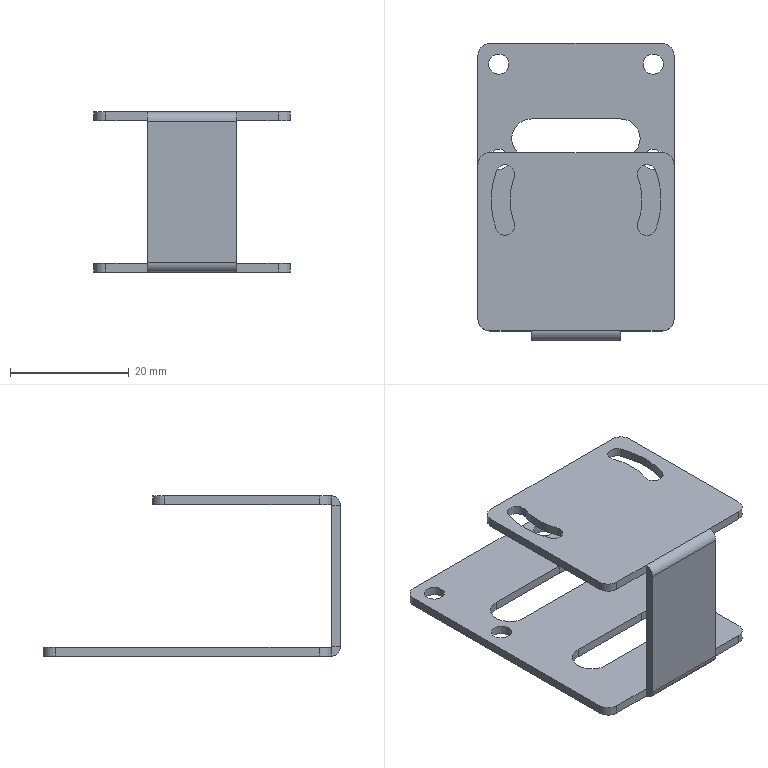Part | STEP file | 1 solid | 64 faces | box 33 x 50 x 27 mm | volume 3903 mm3 | cylinder 38 | plane 26 | commonest cylinder face diameters 3.2 x8 3.4 x8 4 x8 6.6 x6 22.2 x3 28.6 x3